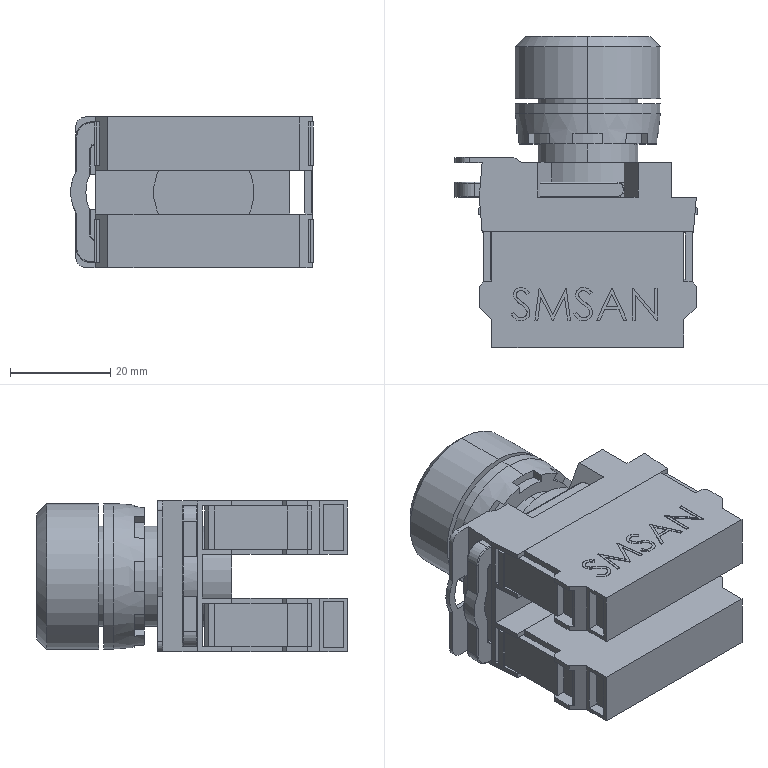Part | STEP file | Yellow button[QG115-A2-10TD╱Y] | 5 solids | 411 faces | box 48.3 x 61.9 x 30.1 mm | volume 44921 mm3 | plane 286 | cylinder 69 | spline 50 | cone 6 | commonest cylinder face diameters 0.4 x20 25 x16 20 x6 2.5 x4 17 x4 29 x4